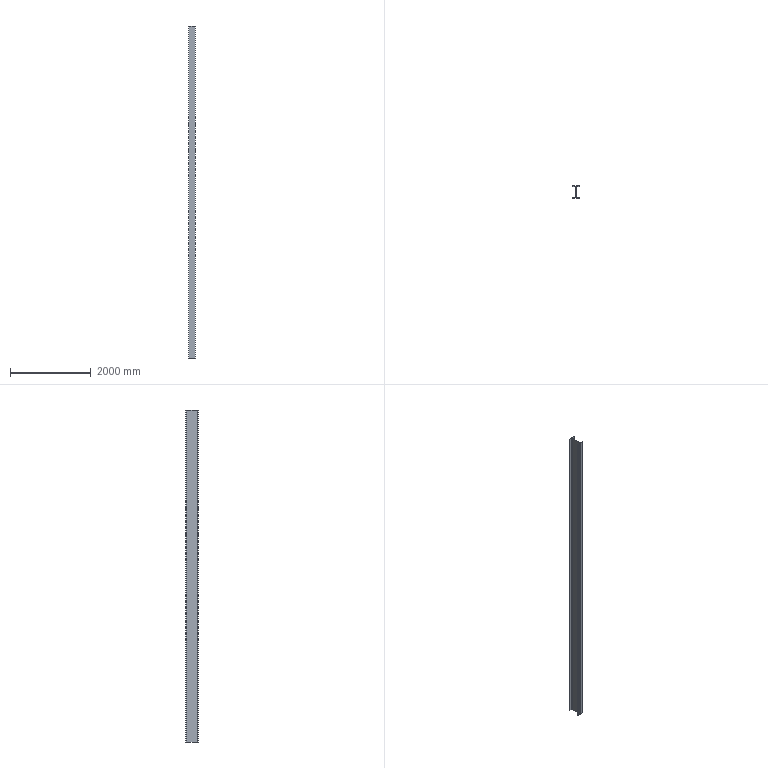Part | SolidWorks | features Extrusion 1 | 1 solid | 18 faces | box 150 x 300 x 8240 mm | volume 38547304 mm3 | plane 14 | cylinder 4 | commonest cylinder face diameters 26 x4
STEP:
#1=CARTESIAN_POINT('',(-75.,9.,0.));
#2=VERTEX_POINT('',#1);
#3=CARTESIAN_POINT('',(-75.,0.,0.));
#4=VERTEX_POINT('',#3);
#5=CARTESIAN_POINT('',(-75.,0.,0.));
#6=DIRECTION('',(0.,-1.,0.));
#7=VECTOR('',#6,1000.);
#8=LINE('',#5,#7);
#9=EDGE_CURVE('',#2,#4,#8,.T.);
#10=ORIENTED_EDGE('',*,*,#9,.T.);
#11=CARTESIAN_POINT('',(-75.,0.,8240.));
#12=VERTEX_POINT('',#11);
#13=CARTESIAN_POINT('',(-75.,0.,8240.));
#14=DIRECTION('',(0.,0.,-1.));
#15=VECTOR('',#14,1000.);
#16=LINE('',#13,#15);
#17=EDGE_CURVE('',#12,#4,#16,.T.);
#18=ORIENTED_EDGE('',*,*,#17,.F.);
#19=CARTESIAN_POINT('',(-75.,9.,8240.));
#20=VERTEX_POINT('',#19);
#21=CARTESIAN_POINT('',(-75.,0.,8240.));
#22=DIRECTION('',(0.,-1.,0.));
#23=VECTOR('',#22,1000.);
#24=LINE('',#21,#23);
#25=EDGE_CURVE('',#20,#12,#24,.T.);
#26=ORIENTED_EDGE('',*,*,#25,.F.);
#27=CARTESIAN_POINT('',(-75.,9.,8240.));
#28=DIRECTION('',(0.,0.,-1.));
#29=VECTOR('',#28,1000.);
#30=LINE('',#27,#29);
#31=EDGE_CURVE('',#20,#2,#30,.T.);
#32=ORIENTED_EDGE('',*,*,#31,.T.);
#33=EDGE_LOOP('',(#10,#18,#26,#32));
#34=FACE_OUTER_BOUND('',#33,.T.);
#35=CARTESIAN_POINT('',(-75.,0.,8240.));
#36=DIRECTION('',(1.,0.,0.));
#37=DIRECTION('',(0.,0.,-1.));
#38=AXIS2_PLACEMENT_3D('',#35,#36,#37);
#39=PLANE('',#38);
#40=ADVANCED_FACE('',(#34),#39,.F.);
#41=CARTESIAN_POINT('',(75.,0.,0.));
#42=VERTEX_POINT('',#41);
#43=CARTESIAN_POINT('',(75.,0.,0.));
#44=DIRECTION('',(1.,0.,0.));
#45=VECTOR('',#44,1000.);
#46=LINE('',#43,#45);
#47=EDGE_CURVE('',#4,#42,#46,.T.);
#48=ORIENTED_EDGE('',*,*,#47,.T.);
#49=CARTESIAN_POINT('',(75.,0.,8240.));
#50=VERTEX_POINT('',#49);
#51=CARTESIAN_POINT('',(75.,0.,8240.));
#52=DIRECTION('',(0.,0.,-1.));
#53=VECTOR('',#52,1000.);
#54=LINE('',#51,#53);
#55=EDGE_CURVE('',#50,#42,#54,.T.);
#56=ORIENTED_EDGE('',*,*,#55,.F.);
#57=CARTESIAN_POINT('',(75.,0.,8240.));
#58=DIRECTION('',(1.,0.,0.));
#59=VECTOR('',#58,1000.);
#60=LINE('',#57,#59);
#61=EDGE_CURVE('',#12,#50,#60,.T.);
#62=ORIENTED_EDGE('',*,*,#61,.F.);
#63=ORIENTED_EDGE('',*,*,#17,.T.);
#64=EDGE_LOOP('',(#48,#56,#62,#63));
#65=FACE_OUTER_BOUND('',#64,.T.);
#66=CARTESIAN_POINT('',(75.,0.,8240.));
#67=DIRECTION('',(0.,1.,0.));
#68=DIRECTION('',(-1.,0.,0.));
#69=AXIS2_PLACEMENT_3D('',#66,#67,#68);
#70=PLANE('',#69);
#71=ADVANCED_FACE('',(#65),#70,.F.);
#72=CARTESIAN_POINT('',(75.,9.,0.));
#73=VERTEX_POINT('',#72);
#74=CARTESIAN_POINT('',(75.,0.,0.));
#75=DIRECTION('',(0.,1.,0.));
#76=VECTOR('',#75,1000.);
#77=LINE('',#74,#76);
#78=EDGE_CURVE('',#42,#73,#77,.T.);
#79=ORIENTED_EDGE('',*,*,#78,.T.);
#80=CARTESIAN_POINT('',(75.,9.,8240.));
#81=VERTEX_POINT('',#80);
#82=CARTESIAN_POINT('',(75.,9.,8240.));
#83=DIRECTION('',(0.,0.,-1.));
#84=VECTOR('',#83,1000.);
#85=LINE('',#82,#84);
#86=EDGE_CURVE('',#81,#73,#85,.T.);
#87=ORIENTED_EDGE('',*,*,#86,.F.);
#88=CARTESIAN_POINT('',(75.,0.,8240.));
#89=DIRECTION('',(0.,1.,0.));
#90=VECTOR('',#89,1000.);
#91=LINE('',#88,#90);
#92=EDGE_CURVE('',#50,#81,#91,.T.);
#93=ORIENTED_EDGE('',*,*,#92,.F.);
#94=ORIENTED_EDGE('',*,*,#55,.T.);
#95=EDGE_LOOP('',(#79,#87,#93,#94));
#96=FACE_OUTER_BOUND('',#95,.T.);
#97=CARTESIAN_POINT('',(75.,0.,8240.));
#98=DIRECTION('',(-1.,0.,0.));
#99=DIRECTION('',(0.,0.,1.));
#100=AXIS2_PLACEMENT_3D('',#97,#98,#99);
#101=PLANE('',#100);
#102=ADVANCED_FACE('',(#96),#101,.F.);
#103=CARTESIAN_POINT('',(16.25,9.,0.));
#104=VERTEX_POINT('',#103);
#105=CARTESIAN_POINT('',(75.,9.,0.));
#106=DIRECTION('',(-1.,0.,0.));
#107=VECTOR('',#106,1000.);
#108=LINE('',#105,#107);
#109=EDGE_CURVE('',#73,#104,#108,.T.);
#110=ORIENTED_EDGE('',*,*,#109,.T.);
#111=CARTESIAN_POINT('',(16.25,9.,8240.));
#112=VERTEX_POINT('',#111);
#113=CARTESIAN_POINT('',(16.25,9.,8240.));
#114=DIRECTION('',(0.,0.,-1.));
#115=VECTOR('',#114,1000.);
#116=LINE('',#113,#115);
#117=EDGE_CURVE('',#112,#104,#116,.T.);
#118=ORIENTED_EDGE('',*,*,#117,.F.);
#119=CARTESIAN_POINT('',(75.,9.,8240.));
#120=DIRECTION('',(-1.,0.,0.));
#121=VECTOR('',#120,1000.);
#122=LINE('',#119,#121);
#123=EDGE_CURVE('',#81,#112,#122,.T.);
#124=ORIENTED_EDGE('',*,*,#123,.F.);
#125=ORIENTED_EDGE('',*,*,#86,.T.);
#126=EDGE_LOOP('',(#110,#118,#124,#125));
#127=FACE_OUTER_BOUND('',#126,.T.);
#128=CARTESIAN_POINT('',(75.,9.,8240.));
#129=DIRECTION('',(0.,-1.,0.));
#130=DIRECTION('',(1.,0.,0.));
#131=AXIS2_PLACEMENT_3D('',#128,#129,#130);
#132=PLANE('',#131);
#133=ADVANCED_FACE('',(#127),#132,.F.);
#134=CARTESIAN_POINT('',(3.25,22.,0.));
#135=VERTEX_POINT('',#134);
#136=CARTESIAN_POINT('',(16.25,22.,0.));
#137=DIRECTION('',(0.,0.,-1.));
#138=DIRECTION('',(-1.,0.,0.));
#139=AXIS2_PLACEMENT_3D('',#136,#137,#138);
#140=CIRCLE('',#139,13.);
#141=EDGE_CURVE('',#104,#135,#140,.T.);
#142=ORIENTED_EDGE('',*,*,#141,.T.);
#143=CARTESIAN_POINT('',(3.25,22.,8240.));
#144=VERTEX_POINT('',#143);
#145=CARTESIAN_POINT('',(3.25,22.,8240.));
#146=DIRECTION('',(0.,0.,-1.));
#147=VECTOR('',#146,1000.);
#148=LINE('',#145,#147);
#149=EDGE_CURVE('',#144,#135,#148,.T.);
#150=ORIENTED_EDGE('',*,*,#149,.F.);
#151=CARTESIAN_POINT('',(16.25,22.,8240.));
#152=DIRECTION('',(0.,0.,-1.));
#153=DIRECTION('',(-1.,0.,0.));
#154=AXIS2_PLACEMENT_3D('',#151,#152,#153);
#155=CIRCLE('',#154,13.);
#156=EDGE_CURVE('',#112,#144,#155,.T.);
#157=ORIENTED_EDGE('',*,*,#156,.F.);
#158=ORIENTED_EDGE('',*,*,#117,.T.);
#159=EDGE_LOOP('',(#142,#150,#157,#158));
#160=FACE_OUTER_BOUND('',#159,.T.);
#161=CARTESIAN_POINT('',(16.25,22.,8240.));
#162=DIRECTION('',(0.,0.,-1.));
#163=DIRECTION('',(-1.,0.,0.));
#164=AXIS2_PLACEMENT_3D('',#161,#162,#163);
#165=CYLINDRICAL_SURFACE('',#164,13.);
#166=ADVANCED_FACE('',(#160),#165,.F.);
#167=CARTESIAN_POINT('',(3.25,278.,0.));
#168=VERTEX_POINT('',#167);
#169=CARTESIAN_POINT('',(3.25,22.,0.));
#170=DIRECTION('',(0.,1.,0.));
#171=VECTOR('',#170,1000.);
#172=LINE('',#169,#171);
#173=EDGE_CURVE('',#135,#168,#172,.T.);
#174=ORIENTED_EDGE('',*,*,#173,.T.);
#175=CARTESIAN_POINT('',(3.25,278.,8240.));
#176=VERTEX_POINT('',#175);
#177=CARTESIAN_POINT('',(3.25,278.,8240.));
#178=DIRECTION('',(0.,0.,-1.));
#179=VECTOR('',#178,1000.);
#180=LINE('',#177,#179);
#181=EDGE_CURVE('',#176,#168,#180,.T.);
#182=ORIENTED_EDGE('',*,*,#181,.F.);
#183=CARTESIAN_POINT('',(3.25,22.,8240.));
#184=DIRECTION('',(0.,1.,0.));
#185=VECTOR('',#184,1000.);
#186=LINE('',#183,#185);
#187=EDGE_CURVE('',#144,#176,#186,.T.);
#188=ORIENTED_EDGE('',*,*,#187,.F.);
#189=ORIENTED_EDGE('',*,*,#149,.T.);
#190=EDGE_LOOP('',(#174,#182,#188,#189));
#191=FACE_OUTER_BOUND('',#190,.T.);
#192=CARTESIAN_POINT('',(3.25,22.,8240.));
#193=DIRECTION('',(-1.,0.,0.));
#194=DIRECTION('',(0.,0.,1.));
#195=AXIS2_PLACEMENT_3D('',#192,#193,#194);
#196=PLANE('',#195);
#197=ADVANCED_FACE('',(#191),#196,.F.);
#198=CARTESIAN_POINT('',(16.25,291.,0.));
#199=VERTEX_POINT('',#198);
#200=CARTESIAN_POINT('',(16.25,278.,0.));
#201=DIRECTION('',(0.,0.,-1.));
#202=DIRECTION('',(-1.,0.,0.));
#203=AXIS2_PLACEMENT_3D('',#200,#201,#202);
#204=CIRCLE('',#203,13.);
#205=EDGE_CURVE('',#168,#199,#204,.T.);
#206=ORIENTED_EDGE('',*,*,#205,.T.);
#207=CARTESIAN_POINT('',(16.25,291.,8240.));
#208=VERTEX_POINT('',#207);
#209=CARTESIAN_POINT('',(16.25,291.,8240.));
#210=DIRECTION('',(0.,0.,-1.));
#211=VECTOR('',#210,1000.);
#212=LINE('',#209,#211);
#213=EDGE_CURVE('',#208,#199,#212,.T.);
#214=ORIENTED_EDGE('',*,*,#213,.F.);
#215=CARTESIAN_POINT('',(16.25,278.,8240.));
#216=DIRECTION('',(0.,0.,-1.));
#217=DIRECTION('',(-1.,0.,0.));
#218=AXIS2_PLACEMENT_3D('',#215,#216,#217);
#219=CIRCLE('',#218,13.);
#220=EDGE_CURVE('',#176,#208,#219,.T.);
#221=ORIENTED_EDGE('',*,*,#220,.F.);
#222=ORIENTED_EDGE('',*,*,#181,.T.);
#223=EDGE_LOOP('',(#206,#214,#221,#222));
#224=FACE_OUTER_BOUND('',#223,.T.);
#225=CARTESIAN_POINT('',(16.25,278.,8240.));
#226=DIRECTION('',(0.,0.,-1.));
#227=DIRECTION('',(-1.,0.,0.));
#228=AXIS2_PLACEMENT_3D('',#225,#226,#227);
#229=CYLINDRICAL_SURFACE('',#228,13.);
#230=ADVANCED_FACE('',(#224),#229,.F.);
#231=CARTESIAN_POINT('',(75.,291.,0.));
#232=VERTEX_POINT('',#231);
#233=CARTESIAN_POINT('',(16.25,291.,0.));
#234=DIRECTION('',(1.,0.,0.));
#235=VECTOR('',#234,1000.);
#236=LINE('',#233,#235);
#237=EDGE_CURVE('',#199,#232,#236,.T.);
#238=ORIENTED_EDGE('',*,*,#237,.T.);
#239=CARTESIAN_POINT('',(75.,291.,8240.));
#240=VERTEX_POINT('',#239);
#241=CARTESIAN_POINT('',(75.,291.,8240.));
#242=DIRECTION('',(0.,0.,-1.));
#243=VECTOR('',#242,1000.);
#244=LINE('',#241,#243);
#245=EDGE_CURVE('',#240,#232,#244,.T.);
#246=ORIENTED_EDGE('',*,*,#245,.F.);
#247=CARTESIAN_POINT('',(16.25,291.,8240.));
#248=DIRECTION('',(1.,0.,0.));
#249=VECTOR('',#248,1000.);
#250=LINE('',#247,#249);
#251=EDGE_CURVE('',#208,#240,#250,.T.);
#252=ORIENTED_EDGE('',*,*,#251,.F.);
#253=ORIENTED_EDGE('',*,*,#213,.T.);
#254=EDGE_LOOP('',(#238,#246,#252,#253));
#255=FACE_OUTER_BOUND('',#254,.T.);
#256=CARTESIAN_POINT('',(16.25,291.,8240.));
#257=DIRECTION('',(0.,1.,0.));
#258=DIRECTION('',(-1.,0.,0.));
#259=AXIS2_PLACEMENT_3D('',#256,#257,#258);
#260=PLANE('',#259);
#261=ADVANCED_FACE('',(#255),#260,.F.);
#262=CARTESIAN_POINT('',(75.,300.,0.));
#263=VERTEX_POINT('',#262);
#264=CARTESIAN_POINT('',(75.,291.,0.));
#265=DIRECTION('',(0.,1.,0.));
#266=VECTOR('',#265,1000.);
#267=LINE('',#264,#266);
#268=EDGE_CURVE('',#232,#263,#267,.T.);
#269=ORIENTED_EDGE('',*,*,#268,.T.);
#270=CARTESIAN_POINT('',(75.,300.,8240.));
#271=VERTEX_POINT('',#270);
#272=CARTESIAN_POINT('',(75.,300.,8240.));
#273=DIRECTION('',(0.,0.,-1.));
#274=VECTOR('',#273,1000.);
#275=LINE('',#272,#274);
#276=EDGE_CURVE('',#271,#263,#275,.T.);
#277=ORIENTED_EDGE('',*,*,#276,.F.);
#278=CARTESIAN_POINT('',(75.,291.,8240.));
#279=DIRECTION('',(0.,1.,0.));
#280=VECTOR('',#279,1000.);
#281=LINE('',#278,#280);
#282=EDGE_CURVE('',#240,#271,#281,.T.);
#283=ORIENTED_EDGE('',*,*,#282,.F.);
#284=ORIENTED_EDGE('',*,*,#245,.T.);
#285=EDGE_LOOP('',(#269,#277,#283,#284));
#286=FACE_OUTER_BOUND('',#285,.T.);
#287=CARTESIAN_POINT('',(75.,291.,8240.));
#288=DIRECTION('',(-1.,0.,0.));
#289=DIRECTION('',(0.,-1.,0.));
#290=AXIS2_PLACEMENT_3D('',#287,#288,#289);
#291=PLANE('',#290);
#292=ADVANCED_FACE('',(#286),#291,.F.);
#293=CARTESIAN_POINT('',(-75.,300.,0.));
#294=VERTEX_POINT('',#293);
#295=CARTESIAN_POINT('',(-75.,300.,0.));
#296=DIRECTION('',(-1.,0.,0.));
#297=VECTOR('',#296,1000.);
#298=LINE('',#295,#297);
#299=EDGE_CURVE('',#263,#294,#298,.T.);
#300=ORIENTED_EDGE('',*,*,#299,.T.);
#301=CARTESIAN_POINT('',(-75.,300.,8240.));
#302=VERTEX_POINT('',#301);
#303=CARTESIAN_POINT('',(-75.,300.,8240.));
#304=DIRECTION('',(0.,0.,-1.));
#305=VECTOR('',#304,1000.);
#306=LINE('',#303,#305);
#307=EDGE_CURVE('',#302,#294,#306,.T.);
#308=ORIENTED_EDGE('',*,*,#307,.F.);
#309=CARTESIAN_POINT('',(-75.,300.,8240.));
#310=DIRECTION('',(-1.,0.,0.));
#311=VECTOR('',#310,1000.);
#312=LINE('',#309,#311);
#313=EDGE_CURVE('',#271,#302,#312,.T.);
#314=ORIENTED_EDGE('',*,*,#313,.F.);
#315=ORIENTED_EDGE('',*,*,#276,.T.);
#316=EDGE_LOOP('',(#300,#308,#314,#315));
#317=FACE_OUTER_BOUND('',#316,.T.);
#318=CARTESIAN_POINT('',(-75.,300.,8240.));
#319=DIRECTION('',(0.,-1.,0.));
#320=DIRECTION('',(0.,0.,-1.));
#321=AXIS2_PLACEMENT_3D('',#318,#319,#320);
#322=PLANE('',#321);
#323=ADVANCED_FACE('',(#317),#322,.F.);
#324=CARTESIAN_POINT('',(-75.,291.,0.));
#325=VERTEX_POINT('',#324);
#326=CARTESIAN_POINT('',(-75.,291.,0.));
#327=DIRECTION('',(0.,-1.,0.));
#328=VECTOR('',#327,1000.);
#329=LINE('',#326,#328);
#330=EDGE_CURVE('',#294,#325,#329,.T.);
#331=ORIENTED_EDGE('',*,*,#330,.T.);
#332=CARTESIAN_POINT('',(-75.,291.,8240.));
#333=VERTEX_POINT('',#332);
#334=CARTESIAN_POINT('',(-75.,291.,8240.));
#335=DIRECTION('',(0.,0.,-1.));
#336=VECTOR('',#335,1000.);
#337=LINE('',#334,#336);
#338=EDGE_CURVE('',#333,#325,#337,.T.);
#339=ORIENTED_EDGE('',*,*,#338,.F.);
#340=CARTESIAN_POINT('',(-75.,291.,8240.));
#341=DIRECTION('',(0.,-1.,0.));
#342=VECTOR('',#341,1000.);
#343=LINE('',#340,#342);
#344=EDGE_CURVE('',#302,#333,#343,.T.);
#345=ORIENTED_EDGE('',*,*,#344,.F.);
#346=ORIENTED_EDGE('',*,*,#307,.T.);
#347=EDGE_LOOP('',(#331,#339,#345,#346));
#348=FACE_OUTER_BOUND('',#347,.T.);
#349=CARTESIAN_POINT('',(-75.,291.,8240.));
#350=DIRECTION('',(1.,0.,0.));
#351=DIRECTION('',(0.,1.,0.));
#352=AXIS2_PLACEMENT_3D('',#349,#350,#351);
#353=PLANE('',#352);
#354=ADVANCED_FACE('',(#348),#353,.F.);
#355=CARTESIAN_POINT('',(-16.25,291.,0.));
#356=VERTEX_POINT('',#355);
#357=CARTESIAN_POINT('',(-16.25,291.,0.));
#358=DIRECTION('',(1.,0.,0.));
#359=VECTOR('',#358,1000.);
#360=LINE('',#357,#359);
#361=EDGE_CURVE('',#325,#356,#360,.T.);
#362=ORIENTED_EDGE('',*,*,#361,.T.);
#363=CARTESIAN_POINT('',(-16.25,291.,8240.));
#364=VERTEX_POINT('',#363);
#365=CARTESIAN_POINT('',(-16.25,291.,8240.));
#366=DIRECTION('',(0.,0.,-1.));
#367=VECTOR('',#366,1000.);
#368=LINE('',#365,#367);
#369=EDGE_CURVE('',#364,#356,#368,.T.);
#370=ORIENTED_EDGE('',*,*,#369,.F.);
#371=CARTESIAN_POINT('',(-16.25,291.,8240.));
#372=DIRECTION('',(1.,0.,0.));
#373=VECTOR('',#372,1000.);
#374=LINE('',#371,#373);
#375=EDGE_CURVE('',#333,#364,#374,.T.);
#376=ORIENTED_EDGE('',*,*,#375,.F.);
#377=ORIENTED_EDGE('',*,*,#338,.T.);
#378=EDGE_LOOP('',(#362,#370,#376,#377));
#379=FACE_OUTER_BOUND('',#378,.T.);
#380=CARTESIAN_POINT('',(-16.25,291.,8240.));
#381=DIRECTION('',(0.,1.,0.));
#382=DIRECTION('',(-1.,0.,0.));
#383=AXIS2_PLACEMENT_3D('',#380,#381,#382);
#384=PLANE('',#383);
#385=ADVANCED_FACE('',(#379),#384,.F.);
#386=CARTESIAN_POINT('',(-3.25,278.,0.));
#387=VERTEX_POINT('',#386);
#388=CARTESIAN_POINT('',(-16.25,278.,0.));
#389=DIRECTION('',(0.,0.,-1.));
#390=DIRECTION('',(1.,0.,0.));
#391=AXIS2_PLACEMENT_3D('',#388,#389,#390);
#392=CIRCLE('',#391,13.);
#393=EDGE_CURVE('',#356,#387,#392,.T.);
#394=ORIENTED_EDGE('',*,*,#393,.T.);
#395=CARTESIAN_POINT('',(-3.25,278.,8240.));
#396=VERTEX_POINT('',#395);
#397=CARTESIAN_POINT('',(-3.25,278.,8240.));
#398=DIRECTION('',(0.,0.,-1.));
#399=VECTOR('',#398,1000.);
#400=LINE('',#397,#399);
#401=EDGE_CURVE('',#396,#387,#400,.T.);
#402=ORIENTED_EDGE('',*,*,#401,.F.);
#403=CARTESIAN_POINT('',(-16.25,278.,8240.));
#404=DIRECTION('',(0.,0.,-1.));
#405=DIRECTION('',(1.,0.,0.));
#406=AXIS2_PLACEMENT_3D('',#403,#404,#405);
#407=CIRCLE('',#406,13.);
#408=EDGE_CURVE('',#364,#396,#407,.T.);
#409=ORIENTED_EDGE('',*,*,#408,.F.);
#410=ORIENTED_EDGE('',*,*,#369,.T.);
#411=EDGE_LOOP('',(#394,#402,#409,#410));
#412=FACE_OUTER_BOUND('',#411,.T.);
#413=CARTESIAN_POINT('',(-16.25,278.,8240.));
#414=DIRECTION('',(0.,0.,-1.));
#415=DIRECTION('',(-1.,0.,0.));
#416=AXIS2_PLACEMENT_3D('',#413,#414,#415);
#417=CYLINDRICAL_SURFACE('',#416,13.);
#418=ADVANCED_FACE('',(#412),#417,.F.);
#419=CARTESIAN_POINT('',(-3.25,22.,0.));
#420=VERTEX_POINT('',#419);
#421=CARTESIAN_POINT('',(-3.25,22.,0.));
#422=DIRECTION('',(0.,-1.,0.));
#423=VECTOR('',#422,1000.);
#424=LINE('',#421,#423);
#425=EDGE_CURVE('',#387,#420,#424,.T.);
#426=ORIENTED_EDGE('',*,*,#425,.T.);
#427=CARTESIAN_POINT('',(-3.25,22.,8240.));
#428=VERTEX_POINT('',#427);
#429=CARTESIAN_POINT('',(-3.25,22.,8240.));
#430=DIRECTION('',(0.,0.,-1.));
#431=VECTOR('',#430,1000.);
#432=LINE('',#429,#431);
#433=EDGE_CURVE('',#428,#420,#432,.T.);
#434=ORIENTED_EDGE('',*,*,#433,.F.);
#435=CARTESIAN_POINT('',(-3.25,22.,8240.));
#436=DIRECTION('',(0.,-1.,0.));
#437=VECTOR('',#436,1000.);
#438=LINE('',#435,#437);
#439=EDGE_CURVE('',#396,#428,#438,.T.);
#440=ORIENTED_EDGE('',*,*,#439,.F.);
#441=ORIENTED_EDGE('',*,*,#401,.T.);
#442=EDGE_LOOP('',(#426,#434,#440,#441));
#443=FACE_OUTER_BOUND('',#442,.T.);
#444=CARTESIAN_POINT('',(-3.25,22.,8240.));
#445=DIRECTION('',(1.,0.,0.));
#446=DIRECTION('',(0.,0.,-1.));
#447=AXIS2_PLACEMENT_3D('',#444,#445,#446);
#448=PLANE('',#447);
#449=ADVANCED_FACE('',(#443),#448,.F.);
#450=CARTESIAN_POINT('',(-16.25,9.,0.));
#451=VERTEX_POINT('',#450);
#452=CARTESIAN_POINT('',(-16.25,22.,0.));
#453=DIRECTION('',(0.,0.,-1.));
#454=DIRECTION('',(-1.,0.,0.));
#455=AXIS2_PLACEMENT_3D('',#452,#453,#454);
#456=CIRCLE('',#455,13.);
#457=EDGE_CURVE('',#420,#451,#456,.T.);
#458=ORIENTED_EDGE('',*,*,#457,.T.);
#459=CARTESIAN_POINT('',(-16.25,9.,8240.));
#460=VERTEX_POINT('',#459);
#461=CARTESIAN_POINT('',(-16.25,9.,8240.));
#462=DIRECTION('',(0.,0.,-1.));
#463=VECTOR('',#462,1000.);
#464=LINE('',#461,#463);
#465=EDGE_CURVE('',#460,#451,#464,.T.);
#466=ORIENTED_EDGE('',*,*,#465,.F.);
#467=CARTESIAN_POINT('',(-16.25,22.,8240.));
#468=DIRECTION('',(0.,0.,-1.));
#469=DIRECTION('',(-1.,0.,0.));
#470=AXIS2_PLACEMENT_3D('',#467,#468,#469);
#471=CIRCLE('',#470,13.);
#472=EDGE_CURVE('',#428,#460,#471,.T.);
#473=ORIENTED_EDGE('',*,*,#472,.F.);
#474=ORIENTED_EDGE('',*,*,#433,.T.);
#475=EDGE_LOOP('',(#458,#466,#473,#474));
#476=FACE_OUTER_BOUND('',#475,.T.);
#477=CARTESIAN_POINT('',(-16.25,22.,8240.));
#478=DIRECTION('',(0.,0.,-1.));
#479=DIRECTION('',(-1.,0.,0.));
#480=AXIS2_PLACEMENT_3D('',#477,#478,#479);
#481=CYLINDRICAL_SURFACE('',#480,13.);
#482=ADVANCED_FACE('',(#476),#481,.F.);
#483=CARTESIAN_POINT('',(-75.,9.,0.));
#484=DIRECTION('',(-1.,0.,0.));
#485=VECTOR('',#484,1000.);
#486=LINE('',#483,#485);
#487=EDGE_CURVE('',#451,#2,#486,.T.);
#488=ORIENTED_EDGE('',*,*,#487,.T.);
#489=ORIENTED_EDGE('',*,*,#31,.F.);
#490=CARTESIAN_POINT('',(-75.,9.,8240.));
#491=DIRECTION('',(-1.,0.,0.));
#492=VECTOR('',#491,1000.);
#493=LINE('',#490,#492);
#494=EDGE_CURVE('',#460,#20,#493,.T.);
#495=ORIENTED_EDGE('',*,*,#494,.F.);
#496=ORIENTED_EDGE('',*,*,#465,.T.);
#497=EDGE_LOOP('',(#488,#489,#495,#496));
#498=FACE_OUTER_BOUND('',#497,.T.);
#499=CARTESIAN_POINT('',(-75.,9.,8240.));
#500=DIRECTION('',(0.,-1.,0.));
#501=DIRECTION('',(1.,0.,0.));
#502=AXIS2_PLACEMENT_3D('',#499,#500,#501);
#503=PLANE('',#502);
#504=ADVANCED_FACE('',(#498),#503,.F.);
#505=ORIENTED_EDGE('',*,*,#25,.T.);
#506=ORIENTED_EDGE('',*,*,#61,.T.);
#507=ORIENTED_EDGE('',*,*,#92,.T.);
#508=ORIENTED_EDGE('',*,*,#123,.T.);
#509=ORIENTED_EDGE('',*,*,#156,.T.);
#510=ORIENTED_EDGE('',*,*,#187,.T.);
#511=ORIENTED_EDGE('',*,*,#220,.T.);
#512=ORIENTED_EDGE('',*,*,#251,.T.);
#513=ORIENTED_EDGE('',*,*,#282,.T.);
#514=ORIENTED_EDGE('',*,*,#313,.T.);
#515=ORIENTED_EDGE('',*,*,#344,.T.);
#516=ORIENTED_EDGE('',*,*,#375,.T.);
#517=ORIENTED_EDGE('',*,*,#408,.T.);
#518=ORIENTED_EDGE('',*,*,#439,.T.);
#519=ORIENTED_EDGE('',*,*,#472,.T.);
#520=ORIENTED_EDGE('',*,*,#494,.T.);
#521=EDGE_LOOP('',(#505,#506,#507,#508,#509,#510,#511,#512,#513,#514,#515,#516,#517,#518,#519,#520));
#522=FACE_OUTER_BOUND('',#521,.T.);
#523=CARTESIAN_POINT('',(-16.25,22.,8240.));
#524=DIRECTION('',(0.,0.,-1.));
#525=DIRECTION('',(-1.,0.,0.));
#526=AXIS2_PLACEMENT_3D('',#523,#524,#525);
#527=PLANE('',#526);
#528=ADVANCED_FACE('',(#522),#527,.F.);
#529=ORIENTED_EDGE('',*,*,#9,.F.);
#530=ORIENTED_EDGE('',*,*,#487,.F.);
#531=ORIENTED_EDGE('',*,*,#457,.F.);
#532=ORIENTED_EDGE('',*,*,#425,.F.);
#533=ORIENTED_EDGE('',*,*,#393,.F.);
#534=ORIENTED_EDGE('',*,*,#361,.F.);
#535=ORIENTED_EDGE('',*,*,#330,.F.);
#536=ORIENTED_EDGE('',*,*,#299,.F.);
#537=ORIENTED_EDGE('',*,*,#268,.F.);
#538=ORIENTED_EDGE('',*,*,#237,.F.);
#539=ORIENTED_EDGE('',*,*,#205,.F.);
#540=ORIENTED_EDGE('',*,*,#173,.F.);
#541=ORIENTED_EDGE('',*,*,#141,.F.);
#542=ORIENTED_EDGE('',*,*,#109,.F.);
#543=ORIENTED_EDGE('',*,*,#78,.F.);
#544=ORIENTED_EDGE('',*,*,#47,.F.);
#545=EDGE_LOOP('',(#529,#530,#531,#532,#533,#534,#535,#536,#537,#538,#539,#540,#541,#542,#543,#544));
#546=FACE_OUTER_BOUND('',#545,.T.);
#547=CARTESIAN_POINT('',(-16.25,22.,0.));
#548=DIRECTION('',(0.,0.,-1.));
#549=DIRECTION('',(-1.,0.,0.));
#550=AXIS2_PLACEMENT_3D('',#547,#548,#549);
#551=PLANE('',#550);
#552=ADVANCED_FACE('',(#546),#551,.T.);
#553=CLOSED_SHELL('',(#40,#71,#102,#133,#166,#197,#230,#261,#292,#323,#354,#385,#418,#449,#482,#504,#528,#552));
#554=MANIFOLD_SOLID_BREP('',#553);
#555=CARTESIAN_POINT('',(0.,0.,0.));
#556=DIRECTION('',(0.,0.,1.));
#557=DIRECTION('',(1.,0.,0.));
#558=AXIS2_PLACEMENT_3D('',#555,#556,#557);
#559=(LENGTH_UNIT()NAMED_UNIT(*)SI_UNIT(.MILLI.,.METRE.));
#560=UNCERTAINTY_MEASURE_WITH_UNIT(LENGTH_MEASURE(0.00001),#559,'','');
#561=(NAMED_UNIT(*)PLANE_ANGLE_UNIT()SI_UNIT($,.RADIAN.));
#562=(NAMED_UNIT(*)SI_UNIT($,.STERADIAN.)SOLID_ANGLE_UNIT());
#563=(GEOMETRIC_REPRESENTATION_CONTEXT(3)GLOBAL_UNCERTAINTY_ASSIGNED_CONTEXT((#560))GLOBAL_UNIT_ASSIGNED_CONTEXT((#559,#561,#562))REPRESENTATION_CONTEXT('',''));
#564=ADVANCED_BREP_SHAPE_REPRESENTATION('',(#554,#558),#563);